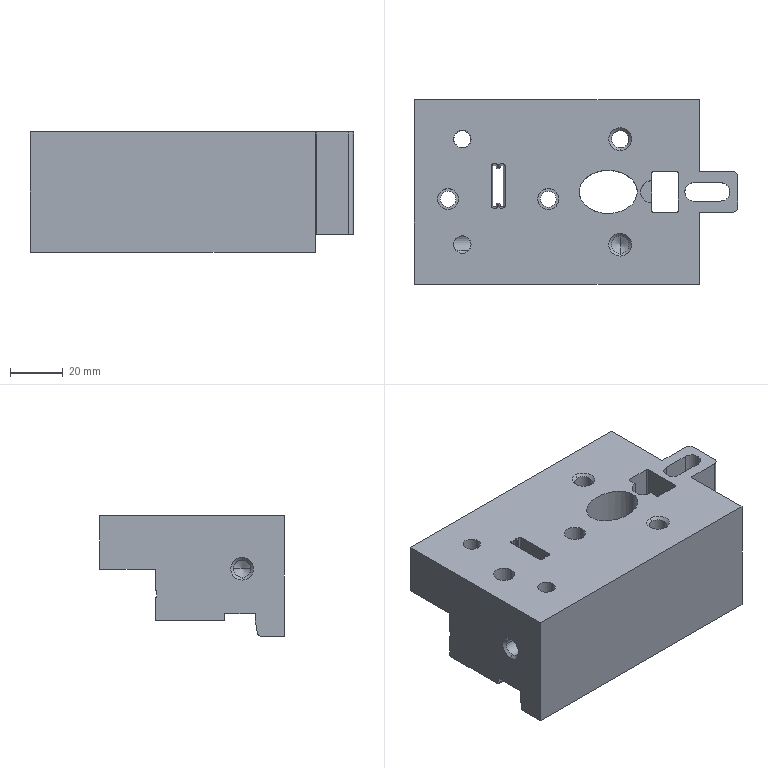Part | STEP file | KHUON AM | 1 solid | 126 faces | box 122.5 x 70 x 45.5 mm | volume 234393 mm3 | plane 54 | cylinder 45 | cone 25 | spline 2 | commonest cylinder face diameters 6.647 x10 1 x7 0.2 x4 0.4 x4 6 x4 8 x4